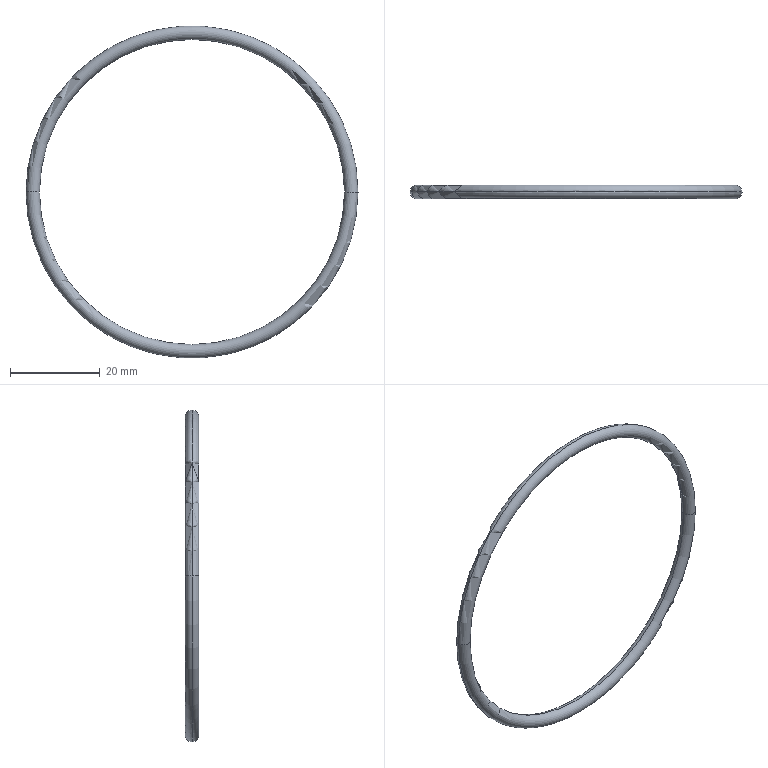Part | SolidWorks | features Revolution 1 | 1 solid | 4 faces | box 74 x 3 x 74 mm | volume 1577 mm3 | torus 4
STEP:
#1=CARTESIAN_POINT('',(-158.531,-104.017,0.));
#2=VERTEX_POINT('',#1);
#3=CARTESIAN_POINT('',(-155.531,-104.017,0.));
#4=VERTEX_POINT('',#3);
#5=CARTESIAN_POINT('',(-157.031,-104.017,0.));
#6=DIRECTION('',(0.,0.,1.));
#7=DIRECTION('',(1.,0.,0.));
#8=AXIS2_PLACEMENT_3D('',#5,#6,#7);
#9=CIRCLE('',#8,1.5);
#10=EDGE_CURVE('',#2,#4,#9,.T.);
#11=ORIENTED_EDGE('',*,*,#10,.F.);
#12=CARTESIAN_POINT('',(-84.531,-104.017,0.));
#13=VERTEX_POINT('',#12);
#14=CARTESIAN_POINT('',(-121.531,-104.017,0.));
#15=DIRECTION('',(0.,-1.,0.));
#16=DIRECTION('',(1.,0.,0.));
#17=AXIS2_PLACEMENT_3D('',#14,#15,#16);
#18=CIRCLE('',#17,37.);
#19=EDGE_CURVE('',#2,#13,#18,.T.);
#20=ORIENTED_EDGE('',*,*,#19,.T.);
#21=CARTESIAN_POINT('',(-87.531,-104.017,0.));
#22=VERTEX_POINT('',#21);
#23=CARTESIAN_POINT('',(-86.031,-104.017,0.));
#24=DIRECTION('',(0.,0.,-1.));
#25=DIRECTION('',(-1.,0.,0.));
#26=AXIS2_PLACEMENT_3D('',#23,#24,#25);
#27=CIRCLE('',#26,1.5);
#28=EDGE_CURVE('',#13,#22,#27,.T.);
#29=ORIENTED_EDGE('',*,*,#28,.T.);
#30=CARTESIAN_POINT('',(-121.531,-104.017,0.));
#31=DIRECTION('',(0.,-1.,0.));
#32=DIRECTION('',(1.,0.,0.));
#33=AXIS2_PLACEMENT_3D('',#30,#31,#32);
#34=CIRCLE('',#33,34.);
#35=EDGE_CURVE('',#4,#22,#34,.T.);
#36=ORIENTED_EDGE('',*,*,#35,.F.);
#37=EDGE_LOOP('',(#11,#20,#29,#36));
#38=FACE_OUTER_BOUND('',#37,.T.);
#39=CARTESIAN_POINT('',(-121.531,-104.017,0.));
#40=DIRECTION('',(0.,-1.,0.));
#41=DIRECTION('',(1.,0.,0.));
#42=AXIS2_PLACEMENT_3D('',#39,#40,#41);
#43=TOROIDAL_SURFACE('',#42,35.5,1.5);
#44=ADVANCED_FACE('',(#38),#43,.T.);
#45=ORIENTED_EDGE('',*,*,#28,.F.);
#46=CARTESIAN_POINT('',(-121.531,-104.017,0.));
#47=DIRECTION('',(0.,-1.,0.));
#48=DIRECTION('',(1.,0.,0.));
#49=AXIS2_PLACEMENT_3D('',#46,#47,#48);
#50=CIRCLE('',#49,37.);
#51=EDGE_CURVE('',#13,#2,#50,.T.);
#52=ORIENTED_EDGE('',*,*,#51,.T.);
#53=ORIENTED_EDGE('',*,*,#10,.T.);
#54=CARTESIAN_POINT('',(-121.531,-104.017,0.));
#55=DIRECTION('',(0.,-1.,0.));
#56=DIRECTION('',(1.,0.,0.));
#57=AXIS2_PLACEMENT_3D('',#54,#55,#56);
#58=CIRCLE('',#57,34.);
#59=EDGE_CURVE('',#22,#4,#58,.T.);
#60=ORIENTED_EDGE('',*,*,#59,.F.);
#61=EDGE_LOOP('',(#45,#52,#53,#60));
#62=FACE_OUTER_BOUND('',#61,.T.);
#63=CARTESIAN_POINT('',(-121.531,-104.017,0.));
#64=DIRECTION('',(0.,-1.,0.));
#65=DIRECTION('',(1.,0.,0.));
#66=AXIS2_PLACEMENT_3D('',#63,#64,#65);
#67=TOROIDAL_SURFACE('',#66,35.5,1.5);
#68=ADVANCED_FACE('',(#62),#67,.T.);
#69=ORIENTED_EDGE('',*,*,#51,.F.);
#70=CARTESIAN_POINT('',(-86.031,-104.017,0.));
#71=DIRECTION('',(0.,0.,-1.));
#72=DIRECTION('',(-1.,0.,0.));
#73=AXIS2_PLACEMENT_3D('',#70,#71,#72);
#74=CIRCLE('',#73,1.5);
#75=EDGE_CURVE('',#22,#13,#74,.T.);
#76=ORIENTED_EDGE('',*,*,#75,.F.);
#77=ORIENTED_EDGE('',*,*,#59,.T.);
#78=CARTESIAN_POINT('',(-157.031,-104.017,0.));
#79=DIRECTION('',(0.,0.,1.));
#80=DIRECTION('',(1.,0.,0.));
#81=AXIS2_PLACEMENT_3D('',#78,#79,#80);
#82=CIRCLE('',#81,1.5);
#83=EDGE_CURVE('',#4,#2,#82,.T.);
#84=ORIENTED_EDGE('',*,*,#83,.T.);
#85=EDGE_LOOP('',(#69,#76,#77,#84));
#86=FACE_OUTER_BOUND('',#85,.T.);
#87=CARTESIAN_POINT('',(-121.531,-104.017,0.));
#88=DIRECTION('',(0.,-1.,0.));
#89=DIRECTION('',(1.,0.,0.));
#90=AXIS2_PLACEMENT_3D('',#87,#88,#89);
#91=TOROIDAL_SURFACE('',#90,35.5,1.5);
#92=ADVANCED_FACE('',(#86),#91,.T.);
#93=ORIENTED_EDGE('',*,*,#19,.F.);
#94=ORIENTED_EDGE('',*,*,#83,.F.);
#95=ORIENTED_EDGE('',*,*,#35,.T.);
#96=ORIENTED_EDGE('',*,*,#75,.T.);
#97=EDGE_LOOP('',(#93,#94,#95,#96));
#98=FACE_OUTER_BOUND('',#97,.T.);
#99=CARTESIAN_POINT('',(-121.531,-104.017,0.));
#100=DIRECTION('',(0.,-1.,0.));
#101=DIRECTION('',(1.,0.,0.));
#102=AXIS2_PLACEMENT_3D('',#99,#100,#101);
#103=TOROIDAL_SURFACE('',#102,35.5,1.5);
#104=ADVANCED_FACE('',(#98),#103,.T.);
#105=CLOSED_SHELL('',(#44,#68,#92,#104));
#106=MANIFOLD_SOLID_BREP('',#105);
#107=CARTESIAN_POINT('',(0.,0.,0.));
#108=DIRECTION('',(0.,0.,1.));
#109=DIRECTION('',(1.,0.,0.));
#110=AXIS2_PLACEMENT_3D('',#107,#108,#109);
#111=(LENGTH_UNIT()NAMED_UNIT(*)SI_UNIT(.MILLI.,.METRE.));
#112=UNCERTAINTY_MEASURE_WITH_UNIT(LENGTH_MEASURE(0.00001),#111,'','');
#113=(NAMED_UNIT(*)PLANE_ANGLE_UNIT()SI_UNIT($,.RADIAN.));
#114=(NAMED_UNIT(*)SI_UNIT($,.STERADIAN.)SOLID_ANGLE_UNIT());
#115=(GEOMETRIC_REPRESENTATION_CONTEXT(3)GLOBAL_UNCERTAINTY_ASSIGNED_CONTEXT((#112))GLOBAL_UNIT_ASSIGNED_CONTEXT((#111,#113,#114))REPRESENTATION_CONTEXT('',''));
#116=ADVANCED_BREP_SHAPE_REPRESENTATION('',(#106,#110),#115);